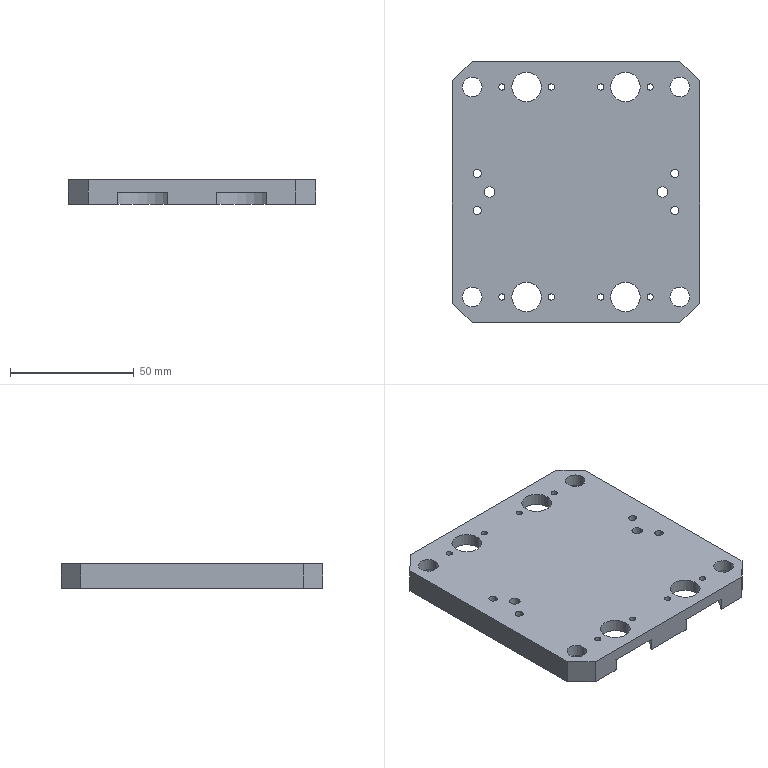Part | SolidWorks | features HoleWzd 4, ICE 3, Chamfer 1, Extrusion 1, MirrorPattern 1 | 1 solid | 82 faces | box 100 x 106 x 10 mm | volume 85872 mm3 | cylinder 64 | plane 18 | commonest cylinder face diameters 2.5 x16 29 x12 3.3 x8 8 x8 12 x8 13 x8